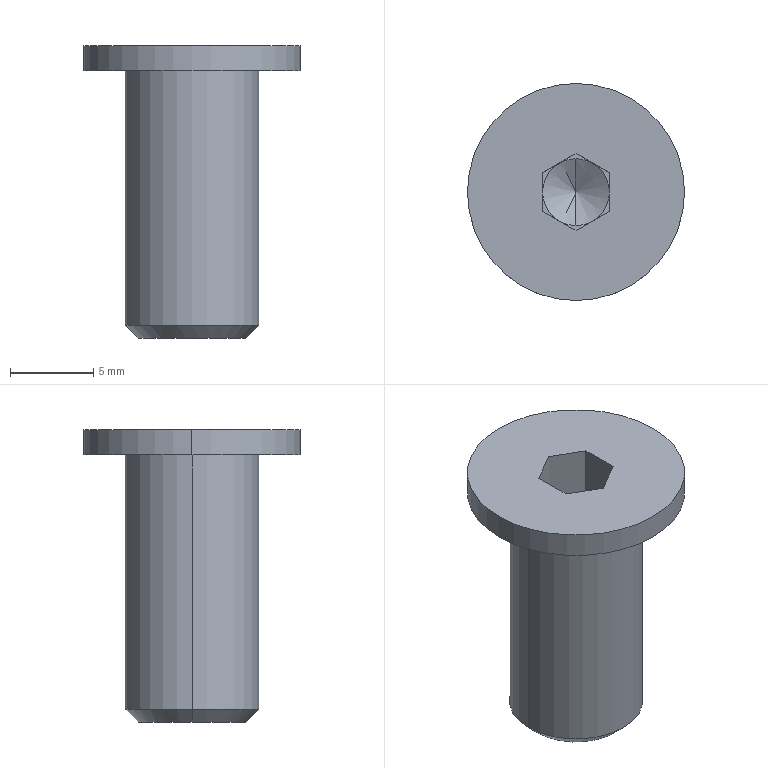Part | SolidWorks | features BaseBody 1 | 1 solid | 23 faces | box 13 x 13 x 17.5 mm | volume 922.307 mm3 | plane 15 | cylinder 4 | cone 4 | commonest cylinder face diameters 8 x2 13 x2
STEP:
#1=CARTESIAN_POINT('',(4.,0.,-15.233));
#2=VERTEX_POINT('',#1);
#3=CARTESIAN_POINT('',(-4.,0.,-15.233));
#4=VERTEX_POINT('',#3);
#5=CARTESIAN_POINT('',(0.,0.,-15.233));
#6=DIRECTION('',(0.,0.,1.));
#7=DIRECTION('',(1.,0.,0.));
#8=AXIS2_PLACEMENT_3D('',#5,#6,#7);
#9=CIRCLE('',#8,4.);
#10=EDGE_CURVE('',#2,#4,#9,.T.);
#11=ORIENTED_EDGE('',*,*,#10,.T.);
#12=CARTESIAN_POINT('',(-4.,0.,0.));
#13=VERTEX_POINT('',#12);
#14=CARTESIAN_POINT('',(-4.,0.,-16.));
#15=DIRECTION('',(0.,0.,1.));
#16=VECTOR('',#15,1000.);
#17=LINE('',#14,#16);
#18=EDGE_CURVE('',#4,#13,#17,.T.);
#19=ORIENTED_EDGE('',*,*,#18,.T.);
#20=CARTESIAN_POINT('',(4.,0.,0.));
#21=VERTEX_POINT('',#20);
#22=CARTESIAN_POINT('',(0.,0.,0.));
#23=DIRECTION('',(0.,0.,-1.));
#24=DIRECTION('',(1.,0.,0.));
#25=AXIS2_PLACEMENT_3D('',#22,#23,#24);
#26=CIRCLE('',#25,4.);
#27=EDGE_CURVE('',#13,#21,#26,.T.);
#28=ORIENTED_EDGE('',*,*,#27,.T.);
#29=CARTESIAN_POINT('',(4.,0.,-16.));
#30=DIRECTION('',(0.,0.,1.));
#31=VECTOR('',#30,1000.);
#32=LINE('',#29,#31);
#33=EDGE_CURVE('',#2,#21,#32,.T.);
#34=ORIENTED_EDGE('',*,*,#33,.F.);
#35=EDGE_LOOP('',(#11,#19,#28,#34));
#36=FACE_OUTER_BOUND('',#35,.T.);
#37=CARTESIAN_POINT('',(0.,0.,-16.));
#38=DIRECTION('',(0.,0.,1.));
#39=DIRECTION('',(1.,0.,0.));
#40=AXIS2_PLACEMENT_3D('',#37,#38,#39);
#41=CYLINDRICAL_SURFACE('',#40,4.);
#42=ADVANCED_FACE('',(#36),#41,.T.);
#43=CARTESIAN_POINT('',(3.233,0.,-16.));
#44=VERTEX_POINT('',#43);
#45=CARTESIAN_POINT('',(-3.233,0.,-16.));
#46=VERTEX_POINT('',#45);
#47=CARTESIAN_POINT('',(0.,0.,-16.));
#48=DIRECTION('',(0.,0.,1.));
#49=DIRECTION('',(1.,0.,0.));
#50=AXIS2_PLACEMENT_3D('',#47,#48,#49);
#51=CIRCLE('',#50,3.233);
#52=EDGE_CURVE('',#44,#46,#51,.T.);
#53=ORIENTED_EDGE('',*,*,#52,.T.);
#54=CARTESIAN_POINT('',(-4.,0.,-15.233));
#55=DIRECTION('',(-0.7071,0.,0.7071));
#56=VECTOR('',#55,1000.);
#57=LINE('',#54,#56);
#58=EDGE_CURVE('',#46,#4,#57,.T.);
#59=ORIENTED_EDGE('',*,*,#58,.T.);
#60=ORIENTED_EDGE('',*,*,#10,.F.);
#61=CARTESIAN_POINT('',(4.,0.,-15.233));
#62=DIRECTION('',(0.7071,0.,0.7071));
#63=VECTOR('',#62,1000.);
#64=LINE('',#61,#63);
#65=EDGE_CURVE('',#44,#2,#64,.T.);
#66=ORIENTED_EDGE('',*,*,#65,.F.);
#67=EDGE_LOOP('',(#53,#59,#60,#66));
#68=FACE_OUTER_BOUND('',#67,.T.);
#69=CARTESIAN_POINT('',(0.,0.,-15.233));
#70=DIRECTION('',(0.,0.,1.));
#71=DIRECTION('',(1.,0.,0.));
#72=AXIS2_PLACEMENT_3D('',#69,#70,#71);
#73=CONICAL_SURFACE('',#72,4.,0.7854);
#74=ADVANCED_FACE('',(#68),#73,.T.);
#75=CARTESIAN_POINT('',(6.5,0.,0.));
#76=VERTEX_POINT('',#75);
#77=CARTESIAN_POINT('',(-6.5,0.,0.));
#78=VERTEX_POINT('',#77);
#79=CARTESIAN_POINT('',(0.,0.,0.));
#80=DIRECTION('',(0.,0.,1.));
#81=DIRECTION('',(1.,0.,0.));
#82=AXIS2_PLACEMENT_3D('',#79,#80,#81);
#83=CIRCLE('',#82,6.5);
#84=EDGE_CURVE('',#76,#78,#83,.T.);
#85=ORIENTED_EDGE('',*,*,#84,.T.);
#86=CARTESIAN_POINT('',(-6.5,0.,1.5));
#87=VERTEX_POINT('',#86);
#88=CARTESIAN_POINT('',(-6.5,0.,0.));
#89=DIRECTION('',(0.,0.,1.));
#90=VECTOR('',#89,1000.);
#91=LINE('',#88,#90);
#92=EDGE_CURVE('',#78,#87,#91,.T.);
#93=ORIENTED_EDGE('',*,*,#92,.T.);
#94=CARTESIAN_POINT('',(6.5,0.,1.5));
#95=VERTEX_POINT('',#94);
#96=CARTESIAN_POINT('',(0.,0.,1.5));
#97=DIRECTION('',(0.,0.,-1.));
#98=DIRECTION('',(1.,0.,0.));
#99=AXIS2_PLACEMENT_3D('',#96,#97,#98);
#100=CIRCLE('',#99,6.5);
#101=EDGE_CURVE('',#87,#95,#100,.T.);
#102=ORIENTED_EDGE('',*,*,#101,.T.);
#103=CARTESIAN_POINT('',(6.5,0.,0.));
#104=DIRECTION('',(0.,0.,1.));
#105=VECTOR('',#104,1000.);
#106=LINE('',#103,#105);
#107=EDGE_CURVE('',#76,#95,#106,.T.);
#108=ORIENTED_EDGE('',*,*,#107,.F.);
#109=EDGE_LOOP('',(#85,#93,#102,#108));
#110=FACE_OUTER_BOUND('',#109,.T.);
#111=CARTESIAN_POINT('',(0.,0.,0.));
#112=DIRECTION('',(0.,0.,1.));
#113=DIRECTION('',(1.,0.,0.));
#114=AXIS2_PLACEMENT_3D('',#111,#112,#113);
#115=CYLINDRICAL_SURFACE('',#114,6.5);
#116=ADVANCED_FACE('',(#110),#115,.T.);
#117=CARTESIAN_POINT('',(0.,0.,-4.655));
#118=VERTEX_POINT('',#117);
#119=CARTESIAN_POINT('',(0.,-2.,-3.5));
#120=VERTEX_POINT('',#119);
#121=CARTESIAN_POINT('',(0.,-2.,-3.5));
#122=DIRECTION('',(0.,-0.866,0.5));
#123=VECTOR('',#122,1000.);
#124=LINE('',#121,#123);
#125=EDGE_CURVE('',#118,#120,#124,.T.);
#126=ORIENTED_EDGE('',*,*,#125,.F.);
#127=CARTESIAN_POINT('',(0.,2.,-3.5));
#128=VERTEX_POINT('',#127);
#129=CARTESIAN_POINT('',(0.,2.,-3.5));
#130=DIRECTION('',(0.,0.866,0.5));
#131=VECTOR('',#130,1000.);
#132=LINE('',#129,#131);
#133=EDGE_CURVE('',#118,#128,#132,.T.);
#134=ORIENTED_EDGE('',*,*,#133,.T.);
#135=CARTESIAN_POINT('',(-1.,1.732,-3.5));
#136=VERTEX_POINT('',#135);
#137=CARTESIAN_POINT('',(0.,0.,-3.5));
#138=DIRECTION('',(0.,0.,-1.));
#139=DIRECTION('',(0.,-1.,0.));
#140=AXIS2_PLACEMENT_3D('',#137,#138,#139);
#141=CIRCLE('',#140,2.);
#142=EDGE_CURVE('',#136,#128,#141,.T.);
#143=ORIENTED_EDGE('',*,*,#142,.F.);
#144=CARTESIAN_POINT('',(-2.,0.,-3.5));
#145=VERTEX_POINT('',#144);
#146=CARTESIAN_POINT('',(0.,0.,-3.5));
#147=DIRECTION('',(0.,0.,-1.));
#148=DIRECTION('',(0.,-1.,0.));
#149=AXIS2_PLACEMENT_3D('',#146,#147,#148);
#150=CIRCLE('',#149,2.);
#151=EDGE_CURVE('',#145,#136,#150,.T.);
#152=ORIENTED_EDGE('',*,*,#151,.F.);
#153=CARTESIAN_POINT('',(-1.,-1.732,-3.5));
#154=VERTEX_POINT('',#153);
#155=CARTESIAN_POINT('',(0.,0.,-3.5));
#156=DIRECTION('',(0.,0.,-1.));
#157=DIRECTION('',(0.,-1.,0.));
#158=AXIS2_PLACEMENT_3D('',#155,#156,#157);
#159=CIRCLE('',#158,2.);
#160=EDGE_CURVE('',#154,#145,#159,.T.);
#161=ORIENTED_EDGE('',*,*,#160,.F.);
#162=CARTESIAN_POINT('',(0.,0.,-3.5));
#163=DIRECTION('',(0.,0.,-1.));
#164=DIRECTION('',(0.,-1.,0.));
#165=AXIS2_PLACEMENT_3D('',#162,#163,#164);
#166=CIRCLE('',#165,2.);
#167=EDGE_CURVE('',#120,#154,#166,.T.);
#168=ORIENTED_EDGE('',*,*,#167,.F.);
#169=EDGE_LOOP('',(#126,#134,#143,#152,#161,#168));
#170=FACE_OUTER_BOUND('',#169,.T.);
#171=CARTESIAN_POINT('',(0.,0.,-3.5));
#172=DIRECTION('',(0.,0.,1.));
#173=DIRECTION('',(0.,-1.,0.));
#174=AXIS2_PLACEMENT_3D('',#171,#172,#173);
#175=CONICAL_SURFACE('',#174,2.,1.047);
#176=ADVANCED_FACE('',(#170),#175,.F.);
#177=ORIENTED_EDGE('',*,*,#18,.F.);
#178=CARTESIAN_POINT('',(0.,0.,-15.233));
#179=DIRECTION('',(0.,0.,1.));
#180=DIRECTION('',(1.,0.,0.));
#181=AXIS2_PLACEMENT_3D('',#178,#179,#180);
#182=CIRCLE('',#181,4.);
#183=EDGE_CURVE('',#4,#2,#182,.T.);
#184=ORIENTED_EDGE('',*,*,#183,.T.);
#185=ORIENTED_EDGE('',*,*,#33,.T.);
#186=CARTESIAN_POINT('',(0.,0.,0.));
#187=DIRECTION('',(0.,0.,-1.));
#188=DIRECTION('',(1.,0.,0.));
#189=AXIS2_PLACEMENT_3D('',#186,#187,#188);
#190=CIRCLE('',#189,4.);
#191=EDGE_CURVE('',#21,#13,#190,.T.);
#192=ORIENTED_EDGE('',*,*,#191,.T.);
#193=EDGE_LOOP('',(#177,#184,#185,#192));
#194=FACE_OUTER_BOUND('',#193,.T.);
#195=CARTESIAN_POINT('',(0.,0.,-16.));
#196=DIRECTION('',(0.,0.,1.));
#197=DIRECTION('',(1.,0.,0.));
#198=AXIS2_PLACEMENT_3D('',#195,#196,#197);
#199=CYLINDRICAL_SURFACE('',#198,4.);
#200=ADVANCED_FACE('',(#194),#199,.T.);
#201=ORIENTED_EDGE('',*,*,#84,.F.);
#202=CARTESIAN_POINT('',(0.,0.,0.));
#203=DIRECTION('',(0.,0.,1.));
#204=DIRECTION('',(1.,0.,0.));
#205=AXIS2_PLACEMENT_3D('',#202,#203,#204);
#206=CIRCLE('',#205,6.5);
#207=EDGE_CURVE('',#78,#76,#206,.T.);
#208=ORIENTED_EDGE('',*,*,#207,.F.);
#209=EDGE_LOOP('',(#201,#208));
#210=FACE_OUTER_BOUND('',#209,.T.);
#211=ORIENTED_EDGE('',*,*,#191,.F.);
#212=ORIENTED_EDGE('',*,*,#27,.F.);
#213=EDGE_LOOP('',(#211,#212));
#214=FACE_BOUND('',#213,.T.);
#215=CARTESIAN_POINT('',(0.,6.5,0.));
#216=DIRECTION('',(0.,0.,1.));
#217=DIRECTION('',(1.,0.,0.));
#218=AXIS2_PLACEMENT_3D('',#215,#216,#217);
#219=PLANE('',#218);
#220=ADVANCED_FACE('',(#210,#214),#219,.F.);
#221=ORIENTED_EDGE('',*,*,#58,.F.);
#222=CARTESIAN_POINT('',(0.,0.,-16.));
#223=DIRECTION('',(0.,0.,1.));
#224=DIRECTION('',(1.,0.,0.));
#225=AXIS2_PLACEMENT_3D('',#222,#223,#224);
#226=CIRCLE('',#225,3.233);
#227=EDGE_CURVE('',#46,#44,#226,.T.);
#228=ORIENTED_EDGE('',*,*,#227,.T.);
#229=ORIENTED_EDGE('',*,*,#65,.T.);
#230=ORIENTED_EDGE('',*,*,#183,.F.);
#231=EDGE_LOOP('',(#221,#228,#229,#230));
#232=FACE_OUTER_BOUND('',#231,.T.);
#233=CARTESIAN_POINT('',(0.,0.,-15.233));
#234=DIRECTION('',(0.,0.,1.));
#235=DIRECTION('',(1.,0.,0.));
#236=AXIS2_PLACEMENT_3D('',#233,#234,#235);
#237=CONICAL_SURFACE('',#236,4.,0.7854);
#238=ADVANCED_FACE('',(#232),#237,.T.);
#239=ORIENTED_EDGE('',*,*,#92,.F.);
#240=ORIENTED_EDGE('',*,*,#207,.T.);
#241=ORIENTED_EDGE('',*,*,#107,.T.);
#242=CARTESIAN_POINT('',(0.,0.,1.5));
#243=DIRECTION('',(0.,0.,-1.));
#244=DIRECTION('',(1.,0.,0.));
#245=AXIS2_PLACEMENT_3D('',#242,#243,#244);
#246=CIRCLE('',#245,6.5);
#247=EDGE_CURVE('',#95,#87,#246,.T.);
#248=ORIENTED_EDGE('',*,*,#247,.T.);
#249=EDGE_LOOP('',(#239,#240,#241,#248));
#250=FACE_OUTER_BOUND('',#249,.T.);
#251=CARTESIAN_POINT('',(0.,0.,0.));
#252=DIRECTION('',(0.,0.,1.));
#253=DIRECTION('',(1.,0.,0.));
#254=AXIS2_PLACEMENT_3D('',#251,#252,#253);
#255=CYLINDRICAL_SURFACE('',#254,6.5);
#256=ADVANCED_FACE('',(#250),#255,.T.);
#257=ORIENTED_EDGE('',*,*,#52,.F.);
#258=ORIENTED_EDGE('',*,*,#227,.F.);
#259=EDGE_LOOP('',(#257,#258));
#260=FACE_OUTER_BOUND('',#259,.T.);
#261=CARTESIAN_POINT('',(0.,3.233,-16.));
#262=DIRECTION('',(0.,0.,1.));
#263=DIRECTION('',(1.,0.,0.));
#264=AXIS2_PLACEMENT_3D('',#261,#262,#263);
#265=PLANE('',#264);
#266=ADVANCED_FACE('',(#260),#265,.F.);
#267=CARTESIAN_POINT('',(-2.,-1.155,1.5));
#268=VERTEX_POINT('',#267);
#269=CARTESIAN_POINT('',(0.,-2.309,1.5));
#270=VERTEX_POINT('',#269);
#271=CARTESIAN_POINT('',(-2.,-1.155,1.5));
#272=DIRECTION('',(0.866,-0.5,0.));
#273=VECTOR('',#272,1000.);
#274=LINE('',#271,#273);
#275=EDGE_CURVE('',#268,#270,#274,.T.);
#276=ORIENTED_EDGE('',*,*,#275,.F.);
#277=CARTESIAN_POINT('',(-2.,1.155,1.5));
#278=VERTEX_POINT('',#277);
#279=CARTESIAN_POINT('',(-2.,0.,1.5));
#280=DIRECTION('',(0.,-1.,0.));
#281=VECTOR('',#280,1000.);
#282=LINE('',#279,#281);
#283=EDGE_CURVE('',#278,#268,#282,.T.);
#284=ORIENTED_EDGE('',*,*,#283,.F.);
#285=CARTESIAN_POINT('',(0.,2.309,1.5));
#286=VERTEX_POINT('',#285);
#287=CARTESIAN_POINT('',(0.,2.309,1.5));
#288=DIRECTION('',(-0.866,-0.5,0.));
#289=VECTOR('',#288,1000.);
#290=LINE('',#287,#289);
#291=EDGE_CURVE('',#286,#278,#290,.T.);
#292=ORIENTED_EDGE('',*,*,#291,.F.);
#293=CARTESIAN_POINT('',(2.,1.155,1.5));
#294=VERTEX_POINT('',#293);
#295=CARTESIAN_POINT('',(2.,1.155,1.5));
#296=DIRECTION('',(-0.866,0.5,0.));
#297=VECTOR('',#296,1000.);
#298=LINE('',#295,#297);
#299=EDGE_CURVE('',#294,#286,#298,.T.);
#300=ORIENTED_EDGE('',*,*,#299,.F.);
#301=CARTESIAN_POINT('',(2.,-1.155,1.5));
#302=VERTEX_POINT('',#301);
#303=CARTESIAN_POINT('',(2.,0.,1.5));
#304=DIRECTION('',(0.,1.,0.));
#305=VECTOR('',#304,1000.);
#306=LINE('',#303,#305);
#307=EDGE_CURVE('',#302,#294,#306,.T.);
#308=ORIENTED_EDGE('',*,*,#307,.F.);
#309=CARTESIAN_POINT('',(0.,-2.309,1.5));
#310=DIRECTION('',(0.866,0.5,0.));
#311=VECTOR('',#310,1000.);
#312=LINE('',#309,#311);
#313=EDGE_CURVE('',#270,#302,#312,.T.);
#314=ORIENTED_EDGE('',*,*,#313,.F.);
#315=EDGE_LOOP('',(#276,#284,#292,#300,#308,#314));
#316=FACE_BOUND('',#315,.T.);
#317=ORIENTED_EDGE('',*,*,#247,.F.);
#318=ORIENTED_EDGE('',*,*,#101,.F.);
#319=EDGE_LOOP('',(#317,#318));
#320=FACE_OUTER_BOUND('',#319,.T.);
#321=CARTESIAN_POINT('',(0.,0.,1.5));
#322=DIRECTION('',(0.,0.,-1.));
#323=DIRECTION('',(-1.,0.,0.));
#324=AXIS2_PLACEMENT_3D('',#321,#322,#323);
#325=PLANE('',#324);
#326=ADVANCED_FACE('',(#316,#320),#325,.F.);
#327=CARTESIAN_POINT('',(2.,-1.155,-3.5));
#328=VERTEX_POINT('',#327);
#329=CARTESIAN_POINT('',(2.,-1.155,-3.5));
#330=DIRECTION('',(0.,0.,1.));
#331=VECTOR('',#330,1000.);
#332=LINE('',#329,#331);
#333=EDGE_CURVE('',#328,#302,#332,.T.);
#334=ORIENTED_EDGE('',*,*,#333,.F.);
#335=CARTESIAN_POINT('',(1.,-1.732,-3.5));
#336=VERTEX_POINT('',#335);
#337=CARTESIAN_POINT('',(1.,-1.732,-3.5));
#338=DIRECTION('',(0.866,0.5,0.));
#339=VECTOR('',#338,1000.);
#340=LINE('',#337,#339);
#341=EDGE_CURVE('',#336,#328,#340,.T.);
#342=ORIENTED_EDGE('',*,*,#341,.F.);
#343=CARTESIAN_POINT('',(0.,-2.309,-3.5));
#344=VERTEX_POINT('',#343);
#345=CARTESIAN_POINT('',(0.,-2.309,-3.5));
#346=DIRECTION('',(0.866,0.5,0.));
#347=VECTOR('',#346,1000.);
#348=LINE('',#345,#347);
#349=EDGE_CURVE('',#344,#336,#348,.T.);
#350=ORIENTED_EDGE('',*,*,#349,.F.);
#351=CARTESIAN_POINT('',(0.,-2.309,-3.5));
#352=DIRECTION('',(0.,0.,-1.));
#353=VECTOR('',#352,1000.);
#354=LINE('',#351,#353);
#355=EDGE_CURVE('',#270,#344,#354,.T.);
#356=ORIENTED_EDGE('',*,*,#355,.F.);
#357=ORIENTED_EDGE('',*,*,#313,.T.);
#358=EDGE_LOOP('',(#334,#342,#350,#356,#357));
#359=FACE_OUTER_BOUND('',#358,.T.);
#360=CARTESIAN_POINT('',(0.,-2.309,-3.5));
#361=DIRECTION('',(0.5,-0.866,0.));
#362=DIRECTION('',(0.866,0.5,0.));
#363=AXIS2_PLACEMENT_3D('',#360,#361,#362);
#364=PLANE('',#363);
#365=ADVANCED_FACE('',(#359),#364,.F.);
#366=ORIENTED_EDGE('',*,*,#355,.T.);
#367=CARTESIAN_POINT('',(-1.,-1.732,-3.5));
#368=DIRECTION('',(0.866,-0.5,0.));
#369=VECTOR('',#368,1000.);
#370=LINE('',#367,#369);
#371=EDGE_CURVE('',#154,#344,#370,.T.);
#372=ORIENTED_EDGE('',*,*,#371,.F.);
#373=CARTESIAN_POINT('',(-2.,-1.155,-3.5));
#374=VERTEX_POINT('',#373);
#375=CARTESIAN_POINT('',(-2.,-1.155,-3.5));
#376=DIRECTION('',(0.866,-0.5,0.));
#377=VECTOR('',#376,1000.);
#378=LINE('',#375,#377);
#379=EDGE_CURVE('',#374,#154,#378,.T.);
#380=ORIENTED_EDGE('',*,*,#379,.F.);
#381=CARTESIAN_POINT('',(-2.,-1.155,-3.5));
#382=DIRECTION('',(0.,0.,-1.));
#383=VECTOR('',#382,1000.);
#384=LINE('',#381,#383);
#385=EDGE_CURVE('',#268,#374,#384,.T.);
#386=ORIENTED_EDGE('',*,*,#385,.F.);
#387=ORIENTED_EDGE('',*,*,#275,.T.);
#388=EDGE_LOOP('',(#366,#372,#380,#386,#387));
#389=FACE_OUTER_BOUND('',#388,.T.);
#390=CARTESIAN_POINT('',(-2.,-1.155,-3.5));
#391=DIRECTION('',(-0.5,-0.866,0.));
#392=DIRECTION('',(0.866,-0.5,0.));
#393=AXIS2_PLACEMENT_3D('',#390,#391,#392);
#394=PLANE('',#393);
#395=ADVANCED_FACE('',(#389),#394,.F.);
#396=ORIENTED_EDGE('',*,*,#385,.T.);
#397=CARTESIAN_POINT('',(-2.,0.,-3.5));
#398=DIRECTION('',(0.,-1.,0.));
#399=VECTOR('',#398,1000.);
#400=LINE('',#397,#399);
#401=EDGE_CURVE('',#145,#374,#400,.T.);
#402=ORIENTED_EDGE('',*,*,#401,.F.);
#403=CARTESIAN_POINT('',(-2.,1.155,-3.5));
#404=VERTEX_POINT('',#403);
#405=CARTESIAN_POINT('',(-2.,0.,-3.5));
#406=DIRECTION('',(0.,-1.,0.));
#407=VECTOR('',#406,1000.);
#408=LINE('',#405,#407);
#409=EDGE_CURVE('',#404,#145,#408,.T.);
#410=ORIENTED_EDGE('',*,*,#409,.F.);
#411=CARTESIAN_POINT('',(-2.,1.155,-3.5));
#412=DIRECTION('',(0.,0.,-1.));
#413=VECTOR('',#412,1000.);
#414=LINE('',#411,#413);
#415=EDGE_CURVE('',#278,#404,#414,.T.);
#416=ORIENTED_EDGE('',*,*,#415,.F.);
#417=ORIENTED_EDGE('',*,*,#283,.T.);
#418=EDGE_LOOP('',(#396,#402,#410,#416,#417));
#419=FACE_OUTER_BOUND('',#418,.T.);
#420=CARTESIAN_POINT('',(-2.,1.155,-3.5));
#421=DIRECTION('',(-1.,0.,0.));
#422=DIRECTION('',(0.,0.,1.));
#423=AXIS2_PLACEMENT_3D('',#420,#421,#422);
#424=PLANE('',#423);
#425=ADVANCED_FACE('',(#419),#424,.F.);
#426=ORIENTED_EDGE('',*,*,#415,.T.);
#427=CARTESIAN_POINT('',(-1.,1.732,-3.5));
#428=DIRECTION('',(-0.866,-0.5,0.));
#429=VECTOR('',#428,1000.);
#430=LINE('',#427,#429);
#431=EDGE_CURVE('',#136,#404,#430,.T.);
#432=ORIENTED_EDGE('',*,*,#431,.F.);
#433=CARTESIAN_POINT('',(0.,2.309,-3.5));
#434=VERTEX_POINT('',#433);
#435=CARTESIAN_POINT('',(0.,2.309,-3.5));
#436=DIRECTION('',(-0.866,-0.5,0.));
#437=VECTOR('',#436,1000.);
#438=LINE('',#435,#437);
#439=EDGE_CURVE('',#434,#136,#438,.T.);
#440=ORIENTED_EDGE('',*,*,#439,.F.);
#441=CARTESIAN_POINT('',(0.,2.309,-3.5));
#442=DIRECTION('',(0.,0.,-1.));
#443=VECTOR('',#442,1000.);
#444=LINE('',#441,#443);
#445=EDGE_CURVE('',#286,#434,#444,.T.);
#446=ORIENTED_EDGE('',*,*,#445,.F.);
#447=ORIENTED_EDGE('',*,*,#291,.T.);
#448=EDGE_LOOP('',(#426,#432,#440,#446,#447));
#449=FACE_OUTER_BOUND('',#448,.T.);
#450=CARTESIAN_POINT('',(0.,2.309,-3.5));
#451=DIRECTION('',(-0.5,0.866,0.));
#452=DIRECTION('',(-0.866,-0.5,0.));
#453=AXIS2_PLACEMENT_3D('',#450,#451,#452);
#454=PLANE('',#453);
#455=ADVANCED_FACE('',(#449),#454,.F.);
#456=ORIENTED_EDGE('',*,*,#445,.T.);
#457=CARTESIAN_POINT('',(1.,1.732,-3.5));
#458=VERTEX_POINT('',#457);
#459=CARTESIAN_POINT('',(1.,1.732,-3.5));
#460=DIRECTION('',(-0.866,0.5,0.));
#461=VECTOR('',#460,1000.);
#462=LINE('',#459,#461);
#463=EDGE_CURVE('',#458,#434,#462,.T.);
#464=ORIENTED_EDGE('',*,*,#463,.F.);
#465=CARTESIAN_POINT('',(2.,1.155,-3.5));
#466=VERTEX_POINT('',#465);
#467=CARTESIAN_POINT('',(2.,1.155,-3.5));
#468=DIRECTION('',(-0.866,0.5,0.));
#469=VECTOR('',#468,1000.);
#470=LINE('',#467,#469);
#471=EDGE_CURVE('',#466,#458,#470,.T.);
#472=ORIENTED_EDGE('',*,*,#471,.F.);
#473=CARTESIAN_POINT('',(2.,1.155,-3.5));
#474=DIRECTION('',(0.,0.,-1.));
#475=VECTOR('',#474,1000.);
#476=LINE('',#473,#475);
#477=EDGE_CURVE('',#294,#466,#476,.T.);
#478=ORIENTED_EDGE('',*,*,#477,.F.);
#479=ORIENTED_EDGE('',*,*,#299,.T.);
#480=EDGE_LOOP('',(#456,#464,#472,#478,#479));
#481=FACE_OUTER_BOUND('',#480,.T.);
#482=CARTESIAN_POINT('',(2.,1.155,-3.5));
#483=DIRECTION('',(0.5,0.866,0.));
#484=DIRECTION('',(-0.866,0.5,0.));
#485=AXIS2_PLACEMENT_3D('',#482,#483,#484);
#486=PLANE('',#485);
#487=ADVANCED_FACE('',(#481),#486,.F.);
#488=ORIENTED_EDGE('',*,*,#477,.T.);
#489=CARTESIAN_POINT('',(2.,0.,-3.5));
#490=VERTEX_POINT('',#489);
#491=CARTESIAN_POINT('',(2.,-1.155,-3.5));
#492=DIRECTION('',(0.,1.,0.));
#493=VECTOR('',#492,1000.);
#494=LINE('',#491,#493);
#495=EDGE_CURVE('',#490,#466,#494,.T.);
#496=ORIENTED_EDGE('',*,*,#495,.F.);
#497=CARTESIAN_POINT('',(2.,0.,-3.5));
#498=DIRECTION('',(0.,1.,0.));
#499=VECTOR('',#498,1000.);
#500=LINE('',#497,#499);
#501=EDGE_CURVE('',#328,#490,#500,.T.);
#502=ORIENTED_EDGE('',*,*,#501,.F.);
#503=ORIENTED_EDGE('',*,*,#333,.T.);
#504=ORIENTED_EDGE('',*,*,#307,.T.);
#505=EDGE_LOOP('',(#488,#496,#502,#503,#504));
#506=FACE_OUTER_BOUND('',#505,.T.);
#507=CARTESIAN_POINT('',(2.,-1.155,-3.5));
#508=DIRECTION('',(1.,0.,0.));
#509=DIRECTION('',(0.,0.,-1.));
#510=AXIS2_PLACEMENT_3D('',#507,#508,#509);
#511=PLANE('',#510);
#512=ADVANCED_FACE('',(#506),#511,.F.);
#513=CARTESIAN_POINT('',(0.,0.,-3.5));
#514=DIRECTION('',(0.,0.,-1.));
#515=DIRECTION('',(0.,-1.,0.));
#516=AXIS2_PLACEMENT_3D('',#513,#514,#515);
#517=CIRCLE('',#516,2.);
#518=EDGE_CURVE('',#458,#490,#517,.T.);
#519=ORIENTED_EDGE('',*,*,#518,.T.);
#520=ORIENTED_EDGE('',*,*,#495,.T.);
#521=ORIENTED_EDGE('',*,*,#471,.T.);
#522=EDGE_LOOP('',(#519,#520,#521));
#523=FACE_OUTER_BOUND('',#522,.T.);
#524=CARTESIAN_POINT('',(0.,0.,-3.5));
#525=DIRECTION('',(0.,0.,1.));
#526=DIRECTION('',(1.,0.,0.));
#527=AXIS2_PLACEMENT_3D('',#524,#525,#526);
#528=PLANE('',#527);
#529=ADVANCED_FACE('',(#523),#528,.T.);
#530=ORIENTED_EDGE('',*,*,#133,.F.);
#531=ORIENTED_EDGE('',*,*,#125,.T.);
#532=CARTESIAN_POINT('',(0.,0.,-3.5));
#533=DIRECTION('',(0.,0.,-1.));
#534=DIRECTION('',(0.,-1.,0.));
#535=AXIS2_PLACEMENT_3D('',#532,#533,#534);
#536=CIRCLE('',#535,2.);
#537=EDGE_CURVE('',#336,#120,#536,.T.);
#538=ORIENTED_EDGE('',*,*,#537,.F.);
#539=CARTESIAN_POINT('',(0.,0.,-3.5));
#540=DIRECTION('',(0.,0.,-1.));
#541=DIRECTION('',(0.,-1.,0.));
#542=AXIS2_PLACEMENT_3D('',#539,#540,#541);
#543=CIRCLE('',#542,2.);
#544=EDGE_CURVE('',#490,#336,#543,.T.);
#545=ORIENTED_EDGE('',*,*,#544,.F.);
#546=ORIENTED_EDGE('',*,*,#518,.F.);
#547=CARTESIAN_POINT('',(0.,0.,-3.5));
#548=DIRECTION('',(0.,0.,-1.));
#549=DIRECTION('',(0.,-1.,0.));
#550=AXIS2_PLACEMENT_3D('',#547,#548,#549);
#551=CIRCLE('',#550,2.);
#552=EDGE_CURVE('',#128,#458,#551,.T.);
#553=ORIENTED_EDGE('',*,*,#552,.F.);
#554=EDGE_LOOP('',(#530,#531,#538,#545,#546,#553));
#555=FACE_OUTER_BOUND('',#554,.T.);
#556=CARTESIAN_POINT('',(0.,0.,-3.5));
#557=DIRECTION('',(0.,0.,1.));
#558=DIRECTION('',(0.,-1.,0.));
#559=AXIS2_PLACEMENT_3D('',#556,#557,#558);
#560=CONICAL_SURFACE('',#559,2.,1.047);
#561=ADVANCED_FACE('',(#555),#560,.F.);
#562=ORIENTED_EDGE('',*,*,#142,.T.);
#563=ORIENTED_EDGE('',*,*,#552,.T.);
#564=ORIENTED_EDGE('',*,*,#463,.T.);
#565=ORIENTED_EDGE('',*,*,#439,.T.);
#566=EDGE_LOOP('',(#562,#563,#564,#565));
#567=FACE_OUTER_BOUND('',#566,.T.);
#568=CARTESIAN_POINT('',(0.,0.,-3.5));
#569=DIRECTION('',(0.,0.,1.));
#570=DIRECTION('',(1.,0.,0.));
#571=AXIS2_PLACEMENT_3D('',#568,#569,#570);
#572=PLANE('',#571);
#573=ADVANCED_FACE('',(#567),#572,.T.);
#574=ORIENTED_EDGE('',*,*,#151,.T.);
#575=ORIENTED_EDGE('',*,*,#431,.T.);
#576=ORIENTED_EDGE('',*,*,#409,.T.);
#577=EDGE_LOOP('',(#574,#575,#576));
#578=FACE_OUTER_BOUND('',#577,.T.);
#579=CARTESIAN_POINT('',(0.,0.,-3.5));
#580=DIRECTION('',(0.,0.,1.));
#581=DIRECTION('',(1.,0.,0.));
#582=AXIS2_PLACEMENT_3D('',#579,#580,#581);
#583=PLANE('',#582);
#584=ADVANCED_FACE('',(#578),#583,.T.);
#585=ORIENTED_EDGE('',*,*,#160,.T.);
#586=ORIENTED_EDGE('',*,*,#401,.T.);
#587=ORIENTED_EDGE('',*,*,#379,.T.);
#588=EDGE_LOOP('',(#585,#586,#587));
#589=FACE_OUTER_BOUND('',#588,.T.);
#590=CARTESIAN_POINT('',(0.,0.,-3.5));
#591=DIRECTION('',(0.,0.,1.));
#592=DIRECTION('',(1.,0.,0.));
#593=AXIS2_PLACEMENT_3D('',#590,#591,#592);
#594=PLANE('',#593);
#595=ADVANCED_FACE('',(#589),#594,.T.);
#596=ORIENTED_EDGE('',*,*,#537,.T.);
#597=ORIENTED_EDGE('',*,*,#167,.T.);
#598=ORIENTED_EDGE('',*,*,#371,.T.);
#599=ORIENTED_EDGE('',*,*,#349,.T.);
#600=EDGE_LOOP('',(#596,#597,#598,#599));
#601=FACE_OUTER_BOUND('',#600,.T.);
#602=CARTESIAN_POINT('',(0.,0.,-3.5));
#603=DIRECTION('',(0.,0.,1.));
#604=DIRECTION('',(1.,0.,0.));
#605=AXIS2_PLACEMENT_3D('',#602,#603,#604);
#606=PLANE('',#605);
#607=ADVANCED_FACE('',(#601),#606,.T.);
#608=ORIENTED_EDGE('',*,*,#544,.T.);
#609=ORIENTED_EDGE('',*,*,#341,.T.);
#610=ORIENTED_EDGE('',*,*,#501,.T.);
#611=EDGE_LOOP('',(#608,#609,#610));
#612=FACE_OUTER_BOUND('',#611,.T.);
#613=CARTESIAN_POINT('',(0.,0.,-3.5));
#614=DIRECTION('',(0.,0.,1.));
#615=DIRECTION('',(1.,0.,0.));
#616=AXIS2_PLACEMENT_3D('',#613,#614,#615);
#617=PLANE('',#616);
#618=ADVANCED_FACE('',(#612),#617,.T.);
#619=CLOSED_SHELL('',(#42,#74,#116,#176,#200,#220,#238,#256,#266,#326,#365,#395,#425,#455,#487,#512,#529,#561,#573,#584,#595,#607,#618));
#620=MANIFOLD_SOLID_BREP('',#619);
#621=CARTESIAN_POINT('',(0.,0.,0.));
#622=DIRECTION('',(0.,0.,1.));
#623=DIRECTION('',(1.,0.,0.));
#624=AXIS2_PLACEMENT_3D('',#621,#622,#623);
#625=(LENGTH_UNIT()NAMED_UNIT(*)SI_UNIT(.MILLI.,.METRE.));
#626=UNCERTAINTY_MEASURE_WITH_UNIT(LENGTH_MEASURE(0.00001),#625,'','');
#627=(NAMED_UNIT(*)PLANE_ANGLE_UNIT()SI_UNIT($,.RADIAN.));
#628=(NAMED_UNIT(*)SI_UNIT($,.STERADIAN.)SOLID_ANGLE_UNIT());
#629=(GEOMETRIC_REPRESENTATION_CONTEXT(3)GLOBAL_UNCERTAINTY_ASSIGNED_CONTEXT((#626))GLOBAL_UNIT_ASSIGNED_CONTEXT((#625,#627,#628))REPRESENTATION_CONTEXT('',''));
#630=ADVANCED_BREP_SHAPE_REPRESENTATION('',(#620,#624),#629);